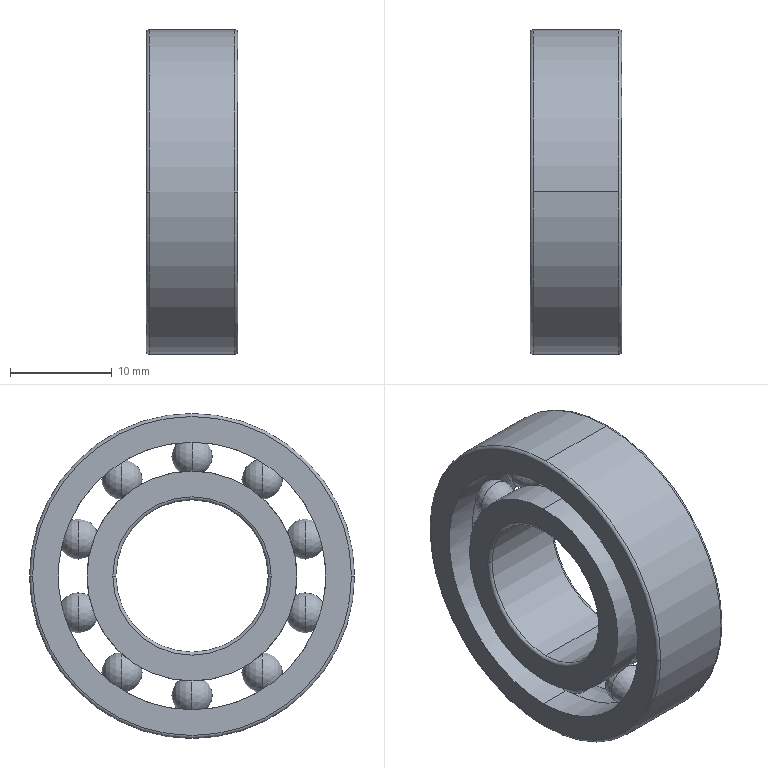Part | NX | 1 solid | 77 faces | box 9 x 32 x 32 mm | volume 3965 mm3 | torus 41 | sphere 20 | cylinder 12 | plane 4 | commonest cylinder face diameters 20.667 x4 26.333 x4 15 x2 32 x2